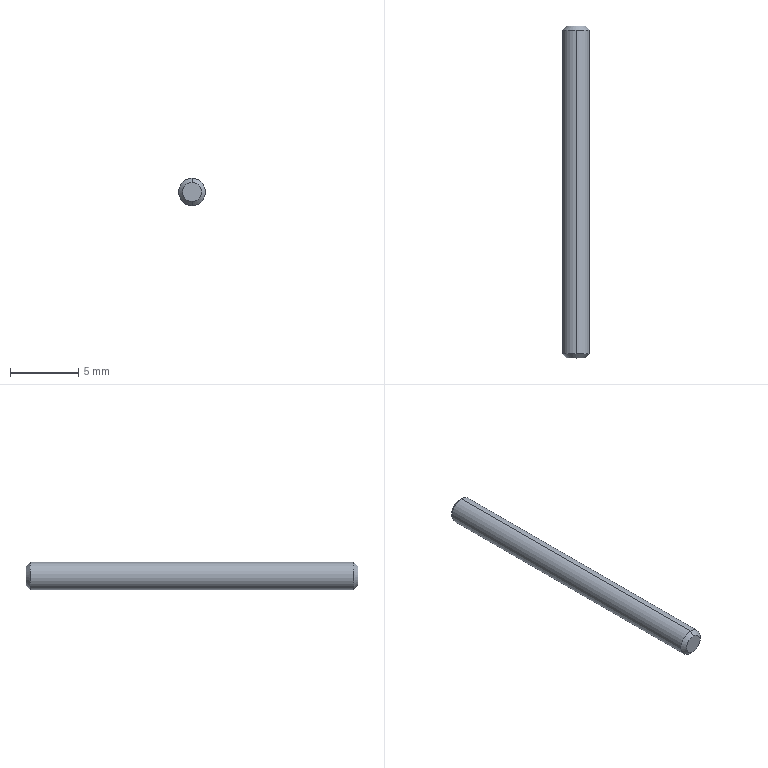Part | SolidWorks | features BaseBody 1 | 1 solid | 8 faces | box 1.99 x 24.35 x 1.99 mm | volume 75.237 mm3 | cone 4 | cylinder 2 | plane 2 | commonest cylinder face diameters 1.99 x2
STEP:
#1=CARTESIAN_POINT('',(2.693,21.195,-12.744));
#2=VERTEX_POINT('',#1);
#3=CARTESIAN_POINT('',(2.693,21.195,-14.734));
#4=VERTEX_POINT('',#3);
#5=CARTESIAN_POINT('',(2.693,21.195,-13.739));
#6=DIRECTION('',(0.,1.,0.));
#7=DIRECTION('',(0.,0.,1.));
#8=AXIS2_PLACEMENT_3D('',#5,#6,#7);
#9=CIRCLE('',#8,0.995);
#10=EDGE_CURVE('',#2,#4,#9,.T.);
#11=ORIENTED_EDGE('',*,*,#10,.T.);
#12=CARTESIAN_POINT('',(2.693,44.95,-14.734));
#13=VERTEX_POINT('',#12);
#14=CARTESIAN_POINT('',(2.693,20.9,-14.734));
#15=DIRECTION('',(0.,1.,0.));
#16=VECTOR('',#15,1000.);
#17=LINE('',#14,#16);
#18=EDGE_CURVE('',#4,#13,#17,.T.);
#19=ORIENTED_EDGE('',*,*,#18,.T.);
#20=CARTESIAN_POINT('',(2.693,44.95,-12.744));
#21=VERTEX_POINT('',#20);
#22=CARTESIAN_POINT('',(2.693,44.95,-13.739));
#23=DIRECTION('',(0.,-1.,0.));
#24=DIRECTION('',(0.,0.,1.));
#25=AXIS2_PLACEMENT_3D('',#22,#23,#24);
#26=CIRCLE('',#25,0.995);
#27=EDGE_CURVE('',#13,#21,#26,.T.);
#28=ORIENTED_EDGE('',*,*,#27,.T.);
#29=CARTESIAN_POINT('',(2.693,20.9,-12.744));
#30=DIRECTION('',(0.,1.,0.));
#31=VECTOR('',#30,1000.);
#32=LINE('',#29,#31);
#33=EDGE_CURVE('',#2,#21,#32,.T.);
#34=ORIENTED_EDGE('',*,*,#33,.F.);
#35=EDGE_LOOP('',(#11,#19,#28,#34));
#36=FACE_OUTER_BOUND('',#35,.T.);
#37=CARTESIAN_POINT('',(2.693,20.9,-13.739));
#38=DIRECTION('',(0.,1.,0.));
#39=DIRECTION('',(0.,0.,1.));
#40=AXIS2_PLACEMENT_3D('',#37,#38,#39);
#41=CYLINDRICAL_SURFACE('',#40,0.995);
#42=ADVANCED_FACE('',(#36),#41,.T.);
#43=CARTESIAN_POINT('',(2.693,45.25,-14.434));
#44=VERTEX_POINT('',#43);
#45=CARTESIAN_POINT('',(2.693,45.25,-13.044));
#46=VERTEX_POINT('',#45);
#47=CARTESIAN_POINT('',(2.693,45.25,-13.739));
#48=DIRECTION('',(0.,-1.,0.));
#49=DIRECTION('',(0.,0.,-1.));
#50=AXIS2_PLACEMENT_3D('',#47,#48,#49);
#51=CIRCLE('',#50,0.695);
#52=EDGE_CURVE('',#44,#46,#51,.T.);
#53=ORIENTED_EDGE('',*,*,#52,.T.);
#54=CARTESIAN_POINT('',(2.693,44.95,-12.744));
#55=DIRECTION('',(0.,-0.7071,0.7071));
#56=VECTOR('',#55,1000.);
#57=LINE('',#54,#56);
#58=EDGE_CURVE('',#46,#21,#57,.T.);
#59=ORIENTED_EDGE('',*,*,#58,.T.);
#60=ORIENTED_EDGE('',*,*,#27,.F.);
#61=CARTESIAN_POINT('',(2.693,44.95,-14.734));
#62=DIRECTION('',(0.,-0.7071,-0.7071));
#63=VECTOR('',#62,1000.);
#64=LINE('',#61,#63);
#65=EDGE_CURVE('',#44,#13,#64,.T.);
#66=ORIENTED_EDGE('',*,*,#65,.F.);
#67=EDGE_LOOP('',(#53,#59,#60,#66));
#68=FACE_OUTER_BOUND('',#67,.T.);
#69=CARTESIAN_POINT('',(2.693,44.95,-13.739));
#70=DIRECTION('',(0.,-1.,0.));
#71=DIRECTION('',(0.,0.,-1.));
#72=AXIS2_PLACEMENT_3D('',#69,#70,#71);
#73=CONICAL_SURFACE('',#72,0.995,0.7854);
#74=ADVANCED_FACE('',(#68),#73,.T.);
#75=CARTESIAN_POINT('',(2.693,20.9,-13.039));
#76=VERTEX_POINT('',#75);
#77=CARTESIAN_POINT('',(2.693,20.9,-14.439));
#78=VERTEX_POINT('',#77);
#79=CARTESIAN_POINT('',(2.693,20.9,-13.739));
#80=DIRECTION('',(0.,1.,0.));
#81=DIRECTION('',(0.,0.,1.));
#82=AXIS2_PLACEMENT_3D('',#79,#80,#81);
#83=CIRCLE('',#82,0.7);
#84=EDGE_CURVE('',#76,#78,#83,.T.);
#85=ORIENTED_EDGE('',*,*,#84,.T.);
#86=CARTESIAN_POINT('',(2.693,21.195,-14.734));
#87=DIRECTION('',(0.,0.7071,-0.7071));
#88=VECTOR('',#87,1000.);
#89=LINE('',#86,#88);
#90=EDGE_CURVE('',#78,#4,#89,.T.);
#91=ORIENTED_EDGE('',*,*,#90,.T.);
#92=ORIENTED_EDGE('',*,*,#10,.F.);
#93=CARTESIAN_POINT('',(2.693,21.195,-12.744));
#94=DIRECTION('',(0.,0.7071,0.7071));
#95=VECTOR('',#94,1000.);
#96=LINE('',#93,#95);
#97=EDGE_CURVE('',#76,#2,#96,.T.);
#98=ORIENTED_EDGE('',*,*,#97,.F.);
#99=EDGE_LOOP('',(#85,#91,#92,#98));
#100=FACE_OUTER_BOUND('',#99,.T.);
#101=CARTESIAN_POINT('',(2.693,21.195,-13.739));
#102=DIRECTION('',(0.,1.,0.));
#103=DIRECTION('',(0.,0.,1.));
#104=AXIS2_PLACEMENT_3D('',#101,#102,#103);
#105=CONICAL_SURFACE('',#104,0.995,0.7854);
#106=ADVANCED_FACE('',(#100),#105,.T.);
#107=ORIENTED_EDGE('',*,*,#18,.F.);
#108=CARTESIAN_POINT('',(2.693,21.195,-13.739));
#109=DIRECTION('',(0.,1.,0.));
#110=DIRECTION('',(0.,0.,1.));
#111=AXIS2_PLACEMENT_3D('',#108,#109,#110);
#112=CIRCLE('',#111,0.995);
#113=EDGE_CURVE('',#4,#2,#112,.T.);
#114=ORIENTED_EDGE('',*,*,#113,.T.);
#115=ORIENTED_EDGE('',*,*,#33,.T.);
#116=CARTESIAN_POINT('',(2.693,44.95,-13.739));
#117=DIRECTION('',(0.,-1.,0.));
#118=DIRECTION('',(0.,0.,1.));
#119=AXIS2_PLACEMENT_3D('',#116,#117,#118);
#120=CIRCLE('',#119,0.995);
#121=EDGE_CURVE('',#21,#13,#120,.T.);
#122=ORIENTED_EDGE('',*,*,#121,.T.);
#123=EDGE_LOOP('',(#107,#114,#115,#122));
#124=FACE_OUTER_BOUND('',#123,.T.);
#125=CARTESIAN_POINT('',(2.693,20.9,-13.739));
#126=DIRECTION('',(0.,1.,0.));
#127=DIRECTION('',(0.,0.,1.));
#128=AXIS2_PLACEMENT_3D('',#125,#126,#127);
#129=CYLINDRICAL_SURFACE('',#128,0.995);
#130=ADVANCED_FACE('',(#124),#129,.T.);
#131=ORIENTED_EDGE('',*,*,#58,.F.);
#132=CARTESIAN_POINT('',(2.693,45.25,-13.739));
#133=DIRECTION('',(0.,-1.,0.));
#134=DIRECTION('',(0.,0.,-1.));
#135=AXIS2_PLACEMENT_3D('',#132,#133,#134);
#136=CIRCLE('',#135,0.695);
#137=EDGE_CURVE('',#46,#44,#136,.T.);
#138=ORIENTED_EDGE('',*,*,#137,.T.);
#139=ORIENTED_EDGE('',*,*,#65,.T.);
#140=ORIENTED_EDGE('',*,*,#121,.F.);
#141=EDGE_LOOP('',(#131,#138,#139,#140));
#142=FACE_OUTER_BOUND('',#141,.T.);
#143=CARTESIAN_POINT('',(2.693,44.95,-13.739));
#144=DIRECTION('',(0.,-1.,0.));
#145=DIRECTION('',(0.,0.,-1.));
#146=AXIS2_PLACEMENT_3D('',#143,#144,#145);
#147=CONICAL_SURFACE('',#146,0.995,0.7854);
#148=ADVANCED_FACE('',(#142),#147,.T.);
#149=ORIENTED_EDGE('',*,*,#90,.F.);
#150=CARTESIAN_POINT('',(2.693,20.9,-13.739));
#151=DIRECTION('',(0.,1.,0.));
#152=DIRECTION('',(0.,0.,1.));
#153=AXIS2_PLACEMENT_3D('',#150,#151,#152);
#154=CIRCLE('',#153,0.7);
#155=EDGE_CURVE('',#78,#76,#154,.T.);
#156=ORIENTED_EDGE('',*,*,#155,.T.);
#157=ORIENTED_EDGE('',*,*,#97,.T.);
#158=ORIENTED_EDGE('',*,*,#113,.F.);
#159=EDGE_LOOP('',(#149,#156,#157,#158));
#160=FACE_OUTER_BOUND('',#159,.T.);
#161=CARTESIAN_POINT('',(2.693,21.195,-13.739));
#162=DIRECTION('',(0.,1.,0.));
#163=DIRECTION('',(0.,0.,1.));
#164=AXIS2_PLACEMENT_3D('',#161,#162,#163);
#165=CONICAL_SURFACE('',#164,0.995,0.7854);
#166=ADVANCED_FACE('',(#160),#165,.T.);
#167=ORIENTED_EDGE('',*,*,#52,.F.);
#168=ORIENTED_EDGE('',*,*,#137,.F.);
#169=EDGE_LOOP('',(#167,#168));
#170=FACE_OUTER_BOUND('',#169,.T.);
#171=CARTESIAN_POINT('',(2.693,45.25,-13.739));
#172=DIRECTION('',(0.,1.,0.));
#173=DIRECTION('',(0.,0.,1.));
#174=AXIS2_PLACEMENT_3D('',#171,#172,#173);
#175=PLANE('',#174);
#176=ADVANCED_FACE('',(#170),#175,.T.);
#177=ORIENTED_EDGE('',*,*,#84,.F.);
#178=ORIENTED_EDGE('',*,*,#155,.F.);
#179=EDGE_LOOP('',(#177,#178));
#180=FACE_OUTER_BOUND('',#179,.T.);
#181=CARTESIAN_POINT('',(2.693,20.9,-13.739));
#182=DIRECTION('',(0.,1.,0.));
#183=DIRECTION('',(0.,0.,1.));
#184=AXIS2_PLACEMENT_3D('',#181,#182,#183);
#185=PLANE('',#184);
#186=ADVANCED_FACE('',(#180),#185,.F.);
#187=CLOSED_SHELL('',(#42,#74,#106,#130,#148,#166,#176,#186));
#188=MANIFOLD_SOLID_BREP('',#187);
#189=CARTESIAN_POINT('',(0.,0.,0.));
#190=DIRECTION('',(0.,0.,1.));
#191=DIRECTION('',(1.,0.,0.));
#192=AXIS2_PLACEMENT_3D('',#189,#190,#191);
#193=(LENGTH_UNIT()NAMED_UNIT(*)SI_UNIT(.MILLI.,.METRE.));
#194=UNCERTAINTY_MEASURE_WITH_UNIT(LENGTH_MEASURE(0.00001),#193,'','');
#195=(NAMED_UNIT(*)PLANE_ANGLE_UNIT()SI_UNIT($,.RADIAN.));
#196=(NAMED_UNIT(*)SI_UNIT($,.STERADIAN.)SOLID_ANGLE_UNIT());
#197=(GEOMETRIC_REPRESENTATION_CONTEXT(3)GLOBAL_UNCERTAINTY_ASSIGNED_CONTEXT((#194))GLOBAL_UNIT_ASSIGNED_CONTEXT((#193,#195,#196))REPRESENTATION_CONTEXT('',''));
#198=ADVANCED_BREP_SHAPE_REPRESENTATION('',(#188,#192),#197);